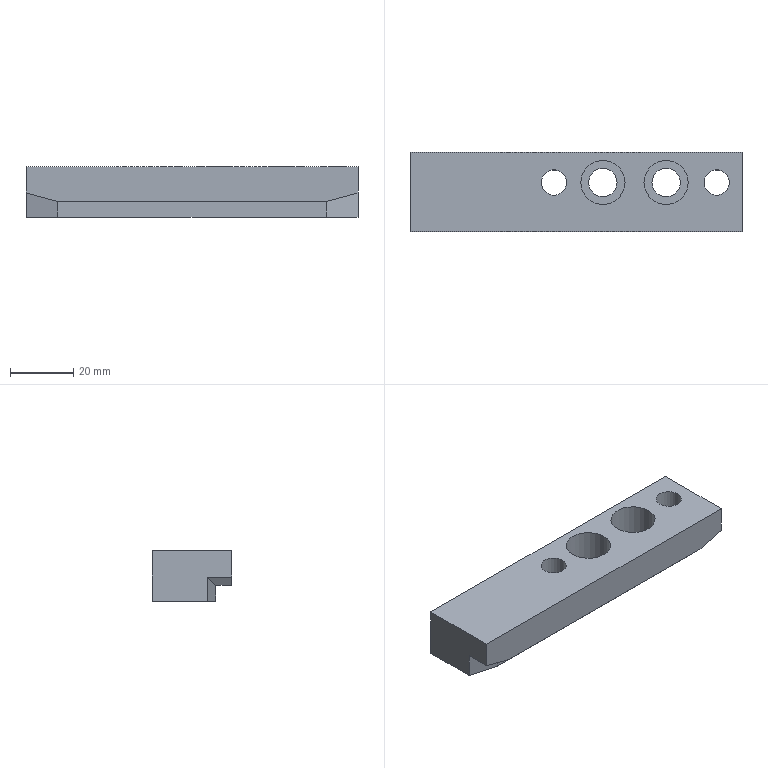Part | STEP file | 1 solid | 20 faces | box 105 x 25 x 16 mm | volume 33608 mm3 | plane 14 | cylinder 6 | commonest cylinder face diameters 8 x2 9 x2 14 x2
STEP:
#1=CARTESIAN_POINT('',(-310.,101.3,3.));
#2=VERTEX_POINT('',#1);
#3=CARTESIAN_POINT('',(-300.,103.98,5.679));
#4=VERTEX_POINT('',#3);
#5=CARTESIAN_POINT('',(-294.77,105.381,7.081));
#6=DIRECTION('',(0.9351,0.2506,0.2506));
#7=VECTOR('',#6,1.);
#8=LINE('',#5,#7);
#9=EDGE_CURVE('',#2,#4,#8,.T.);
#10=ORIENTED_EDGE('',*,*,#9,.T.);
#11=CARTESIAN_POINT('',(-300.,96.3,5.679));
#12=VERTEX_POINT('',#11);
#13=CARTESIAN_POINT('',(-300.,93.8,5.679));
#14=DIRECTION('',(0.,-1.,0.));
#15=VECTOR('',#14,1.);
#16=LINE('',#13,#15);
#17=EDGE_CURVE('',#4,#12,#16,.T.);
#18=ORIENTED_EDGE('',*,*,#17,.T.);
#19=CARTESIAN_POINT('',(-310.,96.3,3.));
#20=VERTEX_POINT('',#19);
#21=CARTESIAN_POINT('',(-302.67,96.3,4.964));
#22=DIRECTION('',(-0.9659,0.,-0.2588));
#23=VECTOR('',#22,1.);
#24=LINE('',#21,#23);
#25=EDGE_CURVE('',#12,#20,#24,.T.);
#26=ORIENTED_EDGE('',*,*,#25,.T.);
#27=CARTESIAN_POINT('',(-310.,101.48,3.));
#28=DIRECTION('',(0.,1.,0.));
#29=VECTOR('',#28,1.);
#30=LINE('',#27,#29);
#31=EDGE_CURVE('',#20,#2,#30,.T.);
#32=ORIENTED_EDGE('',*,*,#31,.T.);
#33=EDGE_LOOP('',(#10,#18,#26,#32));
#34=FACE_OUTER_BOUND('',#33,.T.);
#35=CARTESIAN_POINT('',(-300.,123.8,5.679));
#36=DIRECTION('',(0.2588,0.,-0.9659));
#37=DIRECTION('',(0.9659,0.,0.2588));
#38=AXIS2_PLACEMENT_3D('',#35,#36,#37);
#39=PLANE('',#38);
#40=ADVANCED_FACE('',(#34),#39,.T.);
#41=CARTESIAN_POINT('',(-395.,101.3,3.));
#42=VERTEX_POINT('',#41);
#43=CARTESIAN_POINT('',(-455.,101.3,3.));
#44=DIRECTION('',(-1.,0.,0.));
#45=VECTOR('',#44,1.);
#46=LINE('',#43,#45);
#47=EDGE_CURVE('',#2,#42,#46,.T.);
#48=ORIENTED_EDGE('',*,*,#47,.F.);
#49=ORIENTED_EDGE('',*,*,#31,.F.);
#50=CARTESIAN_POINT('',(-395.,96.3,3.));
#51=VERTEX_POINT('',#50);
#52=CARTESIAN_POINT('',(-365.,96.3,3.));
#53=DIRECTION('',(1.,0.,0.));
#54=VECTOR('',#53,1.);
#55=LINE('',#52,#54);
#56=EDGE_CURVE('',#51,#20,#55,.T.);
#57=ORIENTED_EDGE('',*,*,#56,.F.);
#58=CARTESIAN_POINT('',(-395.,101.48,3.));
#59=DIRECTION('',(0.,1.,0.));
#60=VECTOR('',#59,1.);
#61=LINE('',#58,#60);
#62=EDGE_CURVE('',#51,#42,#61,.T.);
#63=ORIENTED_EDGE('',*,*,#62,.T.);
#64=EDGE_LOOP('',(#48,#49,#57,#63));
#65=FACE_OUTER_BOUND('',#64,.T.);
#66=CARTESIAN_POINT('',(-376.,111.8,3.));
#67=DIRECTION('',(0.,0.,1.));
#68=DIRECTION('',(-1.,0.,0.));
#69=AXIS2_PLACEMENT_3D('',#66,#67,#68);
#70=PLANE('',#69);
#71=ADVANCED_FACE('',(#65),#70,.F.);
#72=CARTESIAN_POINT('',(-405.,103.98,5.679));
#73=VERTEX_POINT('',#72);
#74=CARTESIAN_POINT('',(-410.23,105.381,7.081));
#75=DIRECTION('',(-0.9351,0.2506,0.2506));
#76=VECTOR('',#75,1.);
#77=LINE('',#74,#76);
#78=EDGE_CURVE('',#42,#73,#77,.T.);
#79=ORIENTED_EDGE('',*,*,#78,.F.);
#80=ORIENTED_EDGE('',*,*,#62,.F.);
#81=CARTESIAN_POINT('',(-405.,96.3,5.679));
#82=VERTEX_POINT('',#81);
#83=CARTESIAN_POINT('',(-402.33,96.3,4.964));
#84=DIRECTION('',(0.9659,0.,-0.2588));
#85=VECTOR('',#84,1.);
#86=LINE('',#83,#85);
#87=EDGE_CURVE('',#82,#51,#86,.T.);
#88=ORIENTED_EDGE('',*,*,#87,.F.);
#89=CARTESIAN_POINT('',(-405.,93.8,5.679));
#90=DIRECTION('',(0.,-1.,0.));
#91=VECTOR('',#90,1.);
#92=LINE('',#89,#91);
#93=EDGE_CURVE('',#73,#82,#92,.T.);
#94=ORIENTED_EDGE('',*,*,#93,.F.);
#95=EDGE_LOOP('',(#79,#80,#88,#94));
#96=FACE_OUTER_BOUND('',#95,.T.);
#97=CARTESIAN_POINT('',(-405.,123.8,5.679));
#98=DIRECTION('',(-0.2588,0.,-0.9659));
#99=DIRECTION('',(-0.9659,0.,0.2588));
#100=AXIS2_PLACEMENT_3D('',#97,#98,#99);
#101=PLANE('',#100);
#102=ADVANCED_FACE('',(#96),#101,.T.);
#103=CARTESIAN_POINT('',(-394.998,101.3,-2.));
#104=VERTEX_POINT('',#103);
#105=CARTESIAN_POINT('',(-394.998,101.3,14.));
#106=DIRECTION('',(0.,0.,1.));
#107=VECTOR('',#106,1.);
#108=LINE('',#105,#107);
#109=EDGE_CURVE('',#104,#42,#108,.T.);
#110=ORIENTED_EDGE('',*,*,#109,.T.);
#111=ORIENTED_EDGE('',*,*,#78,.T.);
#112=CARTESIAN_POINT('',(-405.,103.98,-2.));
#113=VERTEX_POINT('',#112);
#114=CARTESIAN_POINT('',(-405.,103.98,-2.));
#115=DIRECTION('',(0.,0.,1.));
#116=VECTOR('',#115,1.);
#117=LINE('',#114,#116);
#118=EDGE_CURVE('',#113,#73,#117,.T.);
#119=ORIENTED_EDGE('',*,*,#118,.F.);
#120=CARTESIAN_POINT('',(-397.317,101.921,-2.));
#121=DIRECTION('',(0.9659,-0.2588,0.));
#122=VECTOR('',#121,1.);
#123=LINE('',#120,#122);
#124=EDGE_CURVE('',#113,#104,#123,.T.);
#125=ORIENTED_EDGE('',*,*,#124,.T.);
#126=EDGE_LOOP('',(#110,#111,#119,#125));
#127=FACE_OUTER_BOUND('',#126,.T.);
#128=CARTESIAN_POINT('',(-395.,101.3,14.));
#129=DIRECTION('',(-0.2588,-0.9659,0.));
#130=DIRECTION('',(0.9659,-0.2588,0.));
#131=AXIS2_PLACEMENT_3D('',#128,#129,#130);
#132=PLANE('',#131);
#133=ADVANCED_FACE('',(#127),#132,.T.);
#134=ORIENTED_EDGE('',*,*,#47,.T.);
#135=ORIENTED_EDGE('',*,*,#109,.F.);
#136=CARTESIAN_POINT('',(-310.002,101.3,-2.));
#137=VERTEX_POINT('',#136);
#138=CARTESIAN_POINT('',(-376.,101.3,-2.));
#139=DIRECTION('',(1.,0.,0.));
#140=VECTOR('',#139,1.);
#141=LINE('',#138,#140);
#142=EDGE_CURVE('',#104,#137,#141,.T.);
#143=ORIENTED_EDGE('',*,*,#142,.T.);
#144=CARTESIAN_POINT('',(-310.002,101.3,14.));
#145=DIRECTION('',(0.,0.,1.));
#146=VECTOR('',#145,1.);
#147=LINE('',#144,#146);
#148=EDGE_CURVE('',#137,#2,#147,.T.);
#149=ORIENTED_EDGE('',*,*,#148,.T.);
#150=EDGE_LOOP('',(#134,#135,#143,#149));
#151=FACE_OUTER_BOUND('',#150,.T.);
#152=CARTESIAN_POINT('',(-455.,101.3,14.));
#153=DIRECTION('',(0.,-1.,0.));
#154=DIRECTION('',(0.,0.,-1.));
#155=AXIS2_PLACEMENT_3D('',#152,#153,#154);
#156=PLANE('',#155);
#157=ADVANCED_FACE('',(#151),#156,.T.);
#158=ORIENTED_EDGE('',*,*,#148,.F.);
#159=CARTESIAN_POINT('',(-300.,103.98,-2.));
#160=VERTEX_POINT('',#159);
#161=CARTESIAN_POINT('',(-307.683,101.921,-2.));
#162=DIRECTION('',(-0.9659,-0.2588,0.));
#163=VECTOR('',#162,1.);
#164=LINE('',#161,#163);
#165=EDGE_CURVE('',#160,#137,#164,.T.);
#166=ORIENTED_EDGE('',*,*,#165,.F.);
#167=CARTESIAN_POINT('',(-300.,103.98,-2.));
#168=DIRECTION('',(0.,0.,1.));
#169=VECTOR('',#168,1.);
#170=LINE('',#167,#169);
#171=EDGE_CURVE('',#160,#4,#170,.T.);
#172=ORIENTED_EDGE('',*,*,#171,.T.);
#173=ORIENTED_EDGE('',*,*,#9,.F.);
#174=EDGE_LOOP('',(#158,#166,#172,#173));
#175=FACE_OUTER_BOUND('',#174,.T.);
#176=CARTESIAN_POINT('',(-310.,101.3,14.));
#177=DIRECTION('',(0.2588,-0.9659,0.));
#178=DIRECTION('',(-0.9659,-0.2588,0.));
#179=AXIS2_PLACEMENT_3D('',#176,#177,#178);
#180=PLANE('',#179);
#181=ADVANCED_FACE('',(#175),#180,.T.);
#182=ORIENTED_EDGE('',*,*,#171,.F.);
#183=CARTESIAN_POINT('',(-300.,121.3,-2.));
#184=VERTEX_POINT('',#183);
#185=CARTESIAN_POINT('',(-300.,123.8,-2.));
#186=DIRECTION('',(0.,-1.,0.));
#187=VECTOR('',#186,1.);
#188=LINE('',#185,#187);
#189=EDGE_CURVE('',#184,#160,#188,.T.);
#190=ORIENTED_EDGE('',*,*,#189,.F.);
#191=CARTESIAN_POINT('',(-300.,121.3,14.));
#192=VERTEX_POINT('',#191);
#193=CARTESIAN_POINT('',(-300.,121.3,-2.));
#194=DIRECTION('',(0.,0.,1.));
#195=VECTOR('',#194,1.);
#196=LINE('',#193,#195);
#197=EDGE_CURVE('',#184,#192,#196,.T.);
#198=ORIENTED_EDGE('',*,*,#197,.T.);
#199=CARTESIAN_POINT('',(-300.,96.3,14.));
#200=VERTEX_POINT('',#199);
#201=CARTESIAN_POINT('',(-300.,123.8,14.));
#202=DIRECTION('',(0.,-1.,0.));
#203=VECTOR('',#202,1.);
#204=LINE('',#201,#203);
#205=EDGE_CURVE('',#192,#200,#204,.T.);
#206=ORIENTED_EDGE('',*,*,#205,.T.);
#207=CARTESIAN_POINT('',(-300.,96.3,-2.));
#208=DIRECTION('',(0.,0.,1.));
#209=VECTOR('',#208,1.);
#210=LINE('',#207,#209);
#211=EDGE_CURVE('',#12,#200,#210,.T.);
#212=ORIENTED_EDGE('',*,*,#211,.F.);
#213=ORIENTED_EDGE('',*,*,#17,.F.);
#214=EDGE_LOOP('',(#182,#190,#198,#206,#212,#213));
#215=FACE_OUTER_BOUND('',#214,.T.);
#216=CARTESIAN_POINT('',(-300.,123.8,-2.));
#217=DIRECTION('',(1.,0.,0.));
#218=DIRECTION('',(0.,0.,1.));
#219=AXIS2_PLACEMENT_3D('',#216,#217,#218);
#220=PLANE('',#219);
#221=ADVANCED_FACE('',(#215),#220,.T.);
#222=CARTESIAN_POINT('',(-405.,96.3,14.));
#223=VERTEX_POINT('',#222);
#224=CARTESIAN_POINT('',(-365.,96.3,14.));
#225=DIRECTION('',(1.,0.,0.));
#226=VECTOR('',#225,1.);
#227=LINE('',#224,#226);
#228=EDGE_CURVE('',#223,#200,#227,.T.);
#229=ORIENTED_EDGE('',*,*,#228,.F.);
#230=CARTESIAN_POINT('',(-405.,96.3,-2.));
#231=DIRECTION('',(0.,0.,1.));
#232=VECTOR('',#231,1.);
#233=LINE('',#230,#232);
#234=EDGE_CURVE('',#82,#223,#233,.T.);
#235=ORIENTED_EDGE('',*,*,#234,.F.);
#236=ORIENTED_EDGE('',*,*,#87,.T.);
#237=ORIENTED_EDGE('',*,*,#56,.T.);
#238=ORIENTED_EDGE('',*,*,#25,.F.);
#239=ORIENTED_EDGE('',*,*,#211,.T.);
#240=EDGE_LOOP('',(#229,#235,#236,#237,#238,#239));
#241=FACE_OUTER_BOUND('',#240,.T.);
#242=CARTESIAN_POINT('',(-365.,96.3,-2.));
#243=DIRECTION('',(0.,-1.,0.));
#244=DIRECTION('',(0.,0.,-1.));
#245=AXIS2_PLACEMENT_3D('',#242,#243,#244);
#246=PLANE('',#245);
#247=ADVANCED_FACE('',(#241),#246,.T.);
#248=ORIENTED_EDGE('',*,*,#118,.T.);
#249=ORIENTED_EDGE('',*,*,#93,.T.);
#250=ORIENTED_EDGE('',*,*,#234,.T.);
#251=CARTESIAN_POINT('',(-405.,121.3,14.));
#252=VERTEX_POINT('',#251);
#253=CARTESIAN_POINT('',(-405.,123.8,14.));
#254=DIRECTION('',(0.,-1.,0.));
#255=VECTOR('',#254,1.);
#256=LINE('',#253,#255);
#257=EDGE_CURVE('',#252,#223,#256,.T.);
#258=ORIENTED_EDGE('',*,*,#257,.F.);
#259=CARTESIAN_POINT('',(-405.,121.3,-2.));
#260=VERTEX_POINT('',#259);
#261=CARTESIAN_POINT('',(-405.,121.3,-2.));
#262=DIRECTION('',(0.,0.,1.));
#263=VECTOR('',#262,1.);
#264=LINE('',#261,#263);
#265=EDGE_CURVE('',#260,#252,#264,.T.);
#266=ORIENTED_EDGE('',*,*,#265,.F.);
#267=CARTESIAN_POINT('',(-405.,123.8,-2.));
#268=DIRECTION('',(0.,-1.,0.));
#269=VECTOR('',#268,1.);
#270=LINE('',#267,#269);
#271=EDGE_CURVE('',#260,#113,#270,.T.);
#272=ORIENTED_EDGE('',*,*,#271,.T.);
#273=EDGE_LOOP('',(#248,#249,#250,#258,#266,#272));
#274=FACE_OUTER_BOUND('',#273,.T.);
#275=CARTESIAN_POINT('',(-405.,123.8,-2.));
#276=DIRECTION('',(-1.,0.,0.));
#277=DIRECTION('',(0.,0.,1.));
#278=AXIS2_PLACEMENT_3D('',#275,#276,#277);
#279=PLANE('',#278);
#280=ADVANCED_FACE('',(#274),#279,.T.);
#281=CARTESIAN_POINT('',(-376.,121.3,-2.));
#282=DIRECTION('',(-1.,0.,0.));
#283=VECTOR('',#282,1.);
#284=LINE('',#281,#283);
#285=EDGE_CURVE('',#184,#260,#284,.T.);
#286=ORIENTED_EDGE('',*,*,#285,.T.);
#287=ORIENTED_EDGE('',*,*,#265,.T.);
#288=CARTESIAN_POINT('',(-376.,121.3,14.));
#289=DIRECTION('',(-1.,0.,0.));
#290=VECTOR('',#289,1.);
#291=LINE('',#288,#290);
#292=EDGE_CURVE('',#192,#252,#291,.T.);
#293=ORIENTED_EDGE('',*,*,#292,.F.);
#294=ORIENTED_EDGE('',*,*,#197,.F.);
#295=EDGE_LOOP('',(#286,#287,#293,#294));
#296=FACE_OUTER_BOUND('',#295,.T.);
#297=CARTESIAN_POINT('',(-465.,121.3,-2.));
#298=DIRECTION('',(0.,1.,0.));
#299=DIRECTION('',(0.,0.,1.));
#300=AXIS2_PLACEMENT_3D('',#297,#298,#299);
#301=PLANE('',#300);
#302=ADVANCED_FACE('',(#296),#301,.T.);
#303=CARTESIAN_POINT('',(-304.,111.8,14.));
#304=VERTEX_POINT('',#303);
#305=CARTESIAN_POINT('',(-308.,111.8,14.));
#306=DIRECTION('',(0.,0.,-1.));
#307=DIRECTION('',(1.,0.,0.));
#308=AXIS2_PLACEMENT_3D('',#305,#306,#307);
#309=CIRCLE('',#308,4.);
#310=EDGE_CURVE('',#304,#304,#309,.T.);
#311=ORIENTED_EDGE('',*,*,#310,.T.);
#312=EDGE_LOOP('',(#311));
#313=FACE_BOUND('',#312,.T.);
#314=CARTESIAN_POINT('',(-355.5,111.8,14.));
#315=VERTEX_POINT('',#314);
#316=CARTESIAN_POINT('',(-359.5,111.8,14.));
#317=DIRECTION('',(0.,0.,-1.));
#318=DIRECTION('',(1.,0.,0.));
#319=AXIS2_PLACEMENT_3D('',#316,#317,#318);
#320=CIRCLE('',#319,4.);
#321=EDGE_CURVE('',#315,#315,#320,.T.);
#322=ORIENTED_EDGE('',*,*,#321,.T.);
#323=EDGE_LOOP('',(#322));
#324=FACE_BOUND('',#323,.T.);
#325=CARTESIAN_POINT('',(-317.,111.8,14.));
#326=VERTEX_POINT('',#325);
#327=CARTESIAN_POINT('',(-324.,111.8,14.));
#328=DIRECTION('',(0.,0.,-1.));
#329=DIRECTION('',(1.,0.,0.));
#330=AXIS2_PLACEMENT_3D('',#327,#328,#329);
#331=CIRCLE('',#330,7.);
#332=EDGE_CURVE('',#326,#326,#331,.T.);
#333=ORIENTED_EDGE('',*,*,#332,.T.);
#334=EDGE_LOOP('',(#333));
#335=FACE_BOUND('',#334,.T.);
#336=CARTESIAN_POINT('',(-337.,111.8,14.));
#337=VERTEX_POINT('',#336);
#338=CARTESIAN_POINT('',(-344.,111.8,14.));
#339=DIRECTION('',(0.,0.,-1.));
#340=DIRECTION('',(1.,0.,0.));
#341=AXIS2_PLACEMENT_3D('',#338,#339,#340);
#342=CIRCLE('',#341,7.);
#343=EDGE_CURVE('',#337,#337,#342,.T.);
#344=ORIENTED_EDGE('',*,*,#343,.T.);
#345=EDGE_LOOP('',(#344));
#346=FACE_BOUND('',#345,.T.);
#347=ORIENTED_EDGE('',*,*,#292,.T.);
#348=ORIENTED_EDGE('',*,*,#257,.T.);
#349=ORIENTED_EDGE('',*,*,#228,.T.);
#350=ORIENTED_EDGE('',*,*,#205,.F.);
#351=EDGE_LOOP('',(#347,#348,#349,#350));
#352=FACE_BOUND('',#351,.T.);
#353=CARTESIAN_POINT('',(-376.,111.8,14.));
#354=DIRECTION('',(0.,0.,1.));
#355=DIRECTION('',(-1.,0.,0.));
#356=AXIS2_PLACEMENT_3D('',#353,#354,#355);
#357=PLANE('',#356);
#358=ADVANCED_FACE('',(#313,#324,#335,#346,#352),#357,.T.);
#359=CARTESIAN_POINT('',(-304.,111.8,-2.));
#360=VERTEX_POINT('',#359);
#361=CARTESIAN_POINT('',(-308.,111.8,-2.));
#362=DIRECTION('',(0.,0.,1.));
#363=DIRECTION('',(1.,0.,0.));
#364=AXIS2_PLACEMENT_3D('',#361,#362,#363);
#365=CIRCLE('',#364,4.);
#366=EDGE_CURVE('',#360,#360,#365,.T.);
#367=ORIENTED_EDGE('',*,*,#366,.T.);
#368=EDGE_LOOP('',(#367));
#369=FACE_BOUND('',#368,.T.);
#370=CARTESIAN_POINT('',(-355.5,111.8,-2.));
#371=VERTEX_POINT('',#370);
#372=CARTESIAN_POINT('',(-359.5,111.8,-2.));
#373=DIRECTION('',(0.,0.,1.));
#374=DIRECTION('',(1.,0.,0.));
#375=AXIS2_PLACEMENT_3D('',#372,#373,#374);
#376=CIRCLE('',#375,4.);
#377=EDGE_CURVE('',#371,#371,#376,.T.);
#378=ORIENTED_EDGE('',*,*,#377,.T.);
#379=EDGE_LOOP('',(#378));
#380=FACE_BOUND('',#379,.T.);
#381=CARTESIAN_POINT('',(-319.5,111.8,-2.));
#382=VERTEX_POINT('',#381);
#383=CARTESIAN_POINT('',(-324.,111.8,-2.));
#384=DIRECTION('',(0.,0.,1.));
#385=DIRECTION('',(1.,0.,0.));
#386=AXIS2_PLACEMENT_3D('',#383,#384,#385);
#387=CIRCLE('',#386,4.5);
#388=EDGE_CURVE('',#382,#382,#387,.T.);
#389=ORIENTED_EDGE('',*,*,#388,.T.);
#390=EDGE_LOOP('',(#389));
#391=FACE_BOUND('',#390,.T.);
#392=CARTESIAN_POINT('',(-339.5,111.8,-2.));
#393=VERTEX_POINT('',#392);
#394=CARTESIAN_POINT('',(-344.,111.8,-2.));
#395=DIRECTION('',(0.,0.,1.));
#396=DIRECTION('',(1.,0.,0.));
#397=AXIS2_PLACEMENT_3D('',#394,#395,#396);
#398=CIRCLE('',#397,4.5);
#399=EDGE_CURVE('',#393,#393,#398,.T.);
#400=ORIENTED_EDGE('',*,*,#399,.T.);
#401=EDGE_LOOP('',(#400));
#402=FACE_BOUND('',#401,.T.);
#403=ORIENTED_EDGE('',*,*,#285,.F.);
#404=ORIENTED_EDGE('',*,*,#189,.T.);
#405=ORIENTED_EDGE('',*,*,#165,.T.);
#406=ORIENTED_EDGE('',*,*,#142,.F.);
#407=ORIENTED_EDGE('',*,*,#124,.F.);
#408=ORIENTED_EDGE('',*,*,#271,.F.);
#409=EDGE_LOOP('',(#403,#404,#405,#406,#407,#408));
#410=FACE_BOUND('',#409,.T.);
#411=CARTESIAN_POINT('',(-376.,111.8,-2.));
#412=DIRECTION('',(0.,0.,1.));
#413=DIRECTION('',(-1.,0.,0.));
#414=AXIS2_PLACEMENT_3D('',#411,#412,#413);
#415=PLANE('',#414);
#416=ADVANCED_FACE('',(#369,#380,#391,#402,#410),#415,.F.);
#417=CARTESIAN_POINT('',(-348.5,111.8,4.));
#418=VERTEX_POINT('',#417);
#419=CARTESIAN_POINT('',(-344.,111.8,4.));
#420=DIRECTION('',(0.,0.,-1.));
#421=DIRECTION('',(-1.,0.,0.));
#422=AXIS2_PLACEMENT_3D('',#419,#420,#421);
#423=CIRCLE('',#422,4.5);
#424=EDGE_CURVE('',#418,#418,#423,.T.);
#425=ORIENTED_EDGE('',*,*,#424,.F.);
#426=EDGE_LOOP('',(#425));
#427=FACE_BOUND('',#426,.T.);
#428=ORIENTED_EDGE('',*,*,#399,.F.);
#429=EDGE_LOOP('',(#428));
#430=FACE_BOUND('',#429,.T.);
#431=CARTESIAN_POINT('',(-344.,111.8,-2.));
#432=DIRECTION('',(0.,0.,1.));
#433=DIRECTION('',(1.,0.,0.));
#434=AXIS2_PLACEMENT_3D('',#431,#432,#433);
#435=CYLINDRICAL_SURFACE('',#434,4.5);
#436=ADVANCED_FACE('',(#427,#430),#435,.F.);
#437=ORIENTED_EDGE('',*,*,#424,.T.);
#438=EDGE_LOOP('',(#437));
#439=FACE_BOUND('',#438,.T.);
#440=CARTESIAN_POINT('',(-337.,111.8,4.));
#441=VERTEX_POINT('',#440);
#442=CARTESIAN_POINT('',(-344.,111.8,4.));
#443=DIRECTION('',(0.,0.,-1.));
#444=DIRECTION('',(1.,0.,0.));
#445=AXIS2_PLACEMENT_3D('',#442,#443,#444);
#446=CIRCLE('',#445,7.);
#447=EDGE_CURVE('',#441,#441,#446,.T.);
#448=ORIENTED_EDGE('',*,*,#447,.F.);
#449=EDGE_LOOP('',(#448));
#450=FACE_BOUND('',#449,.T.);
#451=CARTESIAN_POINT('',(-344.,111.8,4.));
#452=DIRECTION('',(0.,0.,-1.));
#453=DIRECTION('',(-1.,0.,0.));
#454=AXIS2_PLACEMENT_3D('',#451,#452,#453);
#455=PLANE('',#454);
#456=ADVANCED_FACE('',(#439,#450),#455,.F.);
#457=ORIENTED_EDGE('',*,*,#343,.F.);
#458=EDGE_LOOP('',(#457));
#459=FACE_BOUND('',#458,.T.);
#460=ORIENTED_EDGE('',*,*,#447,.T.);
#461=EDGE_LOOP('',(#460));
#462=FACE_BOUND('',#461,.T.);
#463=CARTESIAN_POINT('',(-344.,111.8,4.));
#464=DIRECTION('',(0.,0.,1.));
#465=DIRECTION('',(1.,0.,0.));
#466=AXIS2_PLACEMENT_3D('',#463,#464,#465);
#467=CYLINDRICAL_SURFACE('',#466,7.);
#468=ADVANCED_FACE('',(#459,#462),#467,.F.);
#469=CARTESIAN_POINT('',(-328.5,111.8,4.));
#470=VERTEX_POINT('',#469);
#471=CARTESIAN_POINT('',(-324.,111.8,4.));
#472=DIRECTION('',(0.,0.,-1.));
#473=DIRECTION('',(-1.,0.,0.));
#474=AXIS2_PLACEMENT_3D('',#471,#472,#473);
#475=CIRCLE('',#474,4.5);
#476=EDGE_CURVE('',#470,#470,#475,.T.);
#477=ORIENTED_EDGE('',*,*,#476,.F.);
#478=EDGE_LOOP('',(#477));
#479=FACE_BOUND('',#478,.T.);
#480=ORIENTED_EDGE('',*,*,#388,.F.);
#481=EDGE_LOOP('',(#480));
#482=FACE_BOUND('',#481,.T.);
#483=CARTESIAN_POINT('',(-324.,111.8,-2.));
#484=DIRECTION('',(0.,0.,1.));
#485=DIRECTION('',(1.,0.,0.));
#486=AXIS2_PLACEMENT_3D('',#483,#484,#485);
#487=CYLINDRICAL_SURFACE('',#486,4.5);
#488=ADVANCED_FACE('',(#479,#482),#487,.F.);
#489=ORIENTED_EDGE('',*,*,#476,.T.);
#490=EDGE_LOOP('',(#489));
#491=FACE_BOUND('',#490,.T.);
#492=CARTESIAN_POINT('',(-317.,111.8,4.));
#493=VERTEX_POINT('',#492);
#494=CARTESIAN_POINT('',(-324.,111.8,4.));
#495=DIRECTION('',(0.,0.,-1.));
#496=DIRECTION('',(1.,0.,0.));
#497=AXIS2_PLACEMENT_3D('',#494,#495,#496);
#498=CIRCLE('',#497,7.);
#499=EDGE_CURVE('',#493,#493,#498,.T.);
#500=ORIENTED_EDGE('',*,*,#499,.F.);
#501=EDGE_LOOP('',(#500));
#502=FACE_BOUND('',#501,.T.);
#503=CARTESIAN_POINT('',(-324.,111.8,4.));
#504=DIRECTION('',(0.,0.,-1.));
#505=DIRECTION('',(-1.,0.,0.));
#506=AXIS2_PLACEMENT_3D('',#503,#504,#505);
#507=PLANE('',#506);
#508=ADVANCED_FACE('',(#491,#502),#507,.F.);
#509=ORIENTED_EDGE('',*,*,#332,.F.);
#510=EDGE_LOOP('',(#509));
#511=FACE_BOUND('',#510,.T.);
#512=ORIENTED_EDGE('',*,*,#499,.T.);
#513=EDGE_LOOP('',(#512));
#514=FACE_BOUND('',#513,.T.);
#515=CARTESIAN_POINT('',(-324.,111.8,4.));
#516=DIRECTION('',(0.,0.,1.));
#517=DIRECTION('',(1.,0.,0.));
#518=AXIS2_PLACEMENT_3D('',#515,#516,#517);
#519=CYLINDRICAL_SURFACE('',#518,7.);
#520=ADVANCED_FACE('',(#511,#514),#519,.F.);
#521=ORIENTED_EDGE('',*,*,#321,.F.);
#522=EDGE_LOOP('',(#521));
#523=FACE_BOUND('',#522,.T.);
#524=ORIENTED_EDGE('',*,*,#377,.F.);
#525=EDGE_LOOP('',(#524));
#526=FACE_BOUND('',#525,.T.);
#527=CARTESIAN_POINT('',(-359.5,111.8,-2.));
#528=DIRECTION('',(0.,0.,1.));
#529=DIRECTION('',(1.,0.,0.));
#530=AXIS2_PLACEMENT_3D('',#527,#528,#529);
#531=CYLINDRICAL_SURFACE('',#530,4.);
#532=ADVANCED_FACE('',(#523,#526),#531,.F.);
#533=ORIENTED_EDGE('',*,*,#310,.F.);
#534=EDGE_LOOP('',(#533));
#535=FACE_BOUND('',#534,.T.);
#536=ORIENTED_EDGE('',*,*,#366,.F.);
#537=EDGE_LOOP('',(#536));
#538=FACE_BOUND('',#537,.T.);
#539=CARTESIAN_POINT('',(-308.,111.8,-2.));
#540=DIRECTION('',(0.,0.,1.));
#541=DIRECTION('',(1.,0.,0.));
#542=AXIS2_PLACEMENT_3D('',#539,#540,#541);
#543=CYLINDRICAL_SURFACE('',#542,4.);
#544=ADVANCED_FACE('',(#535,#538),#543,.F.);
#545=CLOSED_SHELL('',(#40,#71,#102,#133,#157,#181,#221,#247,#280,#302,#358,#416,#436,#456,#468,#488,#508,#520,#532,#544));
#546=MANIFOLD_SOLID_BREP('',#545);
#547=(LENGTH_UNIT()NAMED_UNIT(*)SI_UNIT(.MILLI.,.METRE.));
#548=UNCERTAINTY_MEASURE_WITH_UNIT(LENGTH_MEASURE(0.002713),#547,'','');
#549=(NAMED_UNIT(*)PLANE_ANGLE_UNIT()SI_UNIT($,.RADIAN.));
#550=PLANE_ANGLE_MEASURE_WITH_UNIT(PLANE_ANGLE_MEASURE(0.01745),#549);
#551=DIMENSIONAL_EXPONENTS(0.,0.,0.,0.,0.,0.,0.);
#552=(CONVERSION_BASED_UNIT('DEGREE',#550)NAMED_UNIT(#551)PLANE_ANGLE_UNIT());
#553=(NAMED_UNIT(*)SI_UNIT($,.STERADIAN.)SOLID_ANGLE_UNIT());
#554=(GEOMETRIC_REPRESENTATION_CONTEXT(3)GLOBAL_UNCERTAINTY_ASSIGNED_CONTEXT((#548))GLOBAL_UNIT_ASSIGNED_CONTEXT((#547,#552,#553))REPRESENTATION_CONTEXT('',''));
#555=ADVANCED_BREP_SHAPE_REPRESENTATION('',(#546),#554);